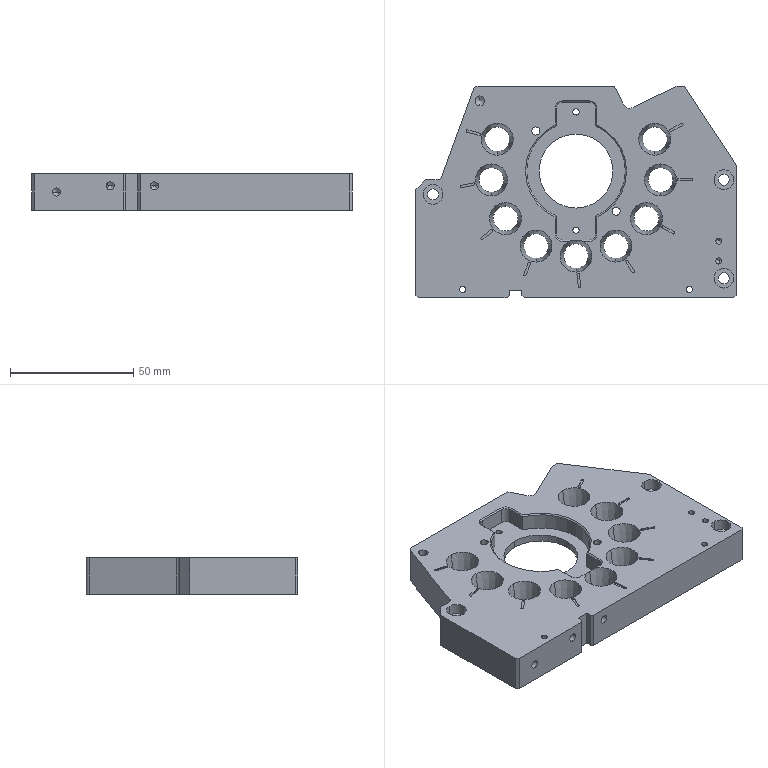NC program | NX | posted with a generic post | part box 130 x 86 x 15 mm
Lines 3649 to 3982 of 51277:
(HOLE_MILLING_COPY , TOOL : D6)
N7254 T06 M6
N7256 G54
N7258 G17 G0 G90 X-1. Y58. B0. C0. S5500 M3
N7260 G43 Z30. H6
N7262 Z0.5
N7264 G94 G3 X-1.5 Y57.5 R0.5 F1500.
N7266 X-1. Y57. R0.5
N7268 X-1. Y57. Z0.4 I0. J1.
N7270 X-1. Y57. Z0.3 I0. J1.
N7272 X-1. Y57. Z0.2 I0. J1.
N7274 X-1. Y57. Z0.1 I0. J1.
N7276 X-1. Y57. Z0. I0. J1.
N7278 X-1. Y57. Z-0.1 I0. J1.
N7280 X-1. Y57. Z-0.2 I0. J1.
N7282 X-1. Y57. Z-0.3 I0. J1.
N7284 X-1. Y57. Z-0.4 I0. J1.
N7286 X-1. Y57. Z-0.5 I0. J1.
N7288 X-1. Y57. Z-0.6 I0. J1.
N7290 X-1. Y57. Z-0.7 I0. J1.
N7292 X-1. Y57. Z-0.8 I0. J1.
N7294 X-1. Y57. Z-0.9 I0. J1.
N7296 X-1. Y57. Z-1. I0. J1.
N7298 X-1. Y57. Z-1.1 I0. J1.
N7300 X-1. Y57. Z-1.2 I0. J1.
N7302 X-1. Y57. Z-1.3 I0. J1.
N7304 X-1. Y57. Z-1.4 I0. J1.
N7306 X-1. Y57. Z-1.5 I0. J1.
N7308 X-1. Y57. Z-1.6 I0. J1.
N7310 X-1. Y57. Z-1.7 I0. J1.
N7312 X-1. Y57. Z-1.8 I0. J1.
N7314 X-1. Y57. Z-1.9 I0. J1.
N7316 X-1. Y57. Z-2. I0. J1.
N7318 X-1. Y57. Z-2.1 I0. J1.
N7320 X-1. Y57. Z-2.2 I0. J1.
N7322 X-1. Y57. Z-2.3 I0. J1.
N7324 X-1. Y57. Z-2.4 I0. J1.
N7326 X-1. Y57. Z-2.5 I0. J1.
N7328 X-1. Y57. Z-2.6 I0. J1.
N7330 X-1. Y57. Z-2.7 I0. J1.
N7332 X-1. Y57. Z-2.8 I0. J1.
N7334 X-1. Y57. Z-2.9 I0. J1.
N7336 X-1. Y57. Z-3. I0. J1.
N7338 X-1. Y57. Z-3.1 I0. J1.
N7340 X-1. Y57. Z-3.2 I0. J1.
N7342 X-1. Y57. Z-3.3 I0. J1.
N7344 X-1. Y57. Z-3.4 I0. J1.
N7346 X-1. Y57. Z-3.5 I0. J1.
N7348 X-1. Y57. Z-3.6 I0. J1.
N7350 X-1. Y57. Z-3.7 I0. J1.
N7352 X-1. Y57. Z-3.8 I0. J1.
N7354 X-1. Y57. Z-3.9 I0. J1.
N7356 X-1. Y57. Z-4. I0. J1.
N7358 X-1. Y57. Z-4.1 I0. J1.
N7360 X-1. Y57. Z-4.2 I0. J1.
N7362 X-1. Y57. Z-4.3 I0. J1.
N7364 X-1. Y57. Z-4.4 I0. J1.
N7366 X-1. Y57. Z-4.5 I0. J1.
N7368 X-1. Y57. Z-4.6 I0. J1.
N7370 X0. Y58. R1.
N7372 X-1. Y57. R-1.
N7374 X-0.5 Y57.5 R0.5
N7376 X-1. Y58. R0.5
N7378 G0 Z30.
N7380 X5. Y-60.
N7382 Z0.5
N7384 G3 X4.5 Y-60.5 R0.5
N7386 X5. Y-61. R0.5
N7388 X5. Y-61. Z0.4 I0. J1.
N7390 X5. Y-61. Z0.3 I0. J1.
N7392 X5. Y-61. Z0.2 I0. J1.
N7394 X5. Y-61. Z0.1 I0. J1.
N7396 X5. Y-61. Z0. I0. J1.
N7398 X5. Y-61. Z-0.1 I0. J1.
N7400 X5. Y-61. Z-0.2 I0. J1.
N7402 X5. Y-61. Z-0.3 I0. J1.
N7404 X5. Y-61. Z-0.4 I0. J1.
N7406 X5. Y-61. Z-0.5 I0. J1.
N7408 X5. Y-61. Z-0.6 I0. J1.
N7410 X5. Y-61. Z-0.7 I0. J1.
N7412 X5. Y-61. Z-0.8 I0. J1.
N7414 X5. Y-61. Z-0.9 I0. J1.
N7416 X5. Y-61. Z-1. I0. J1.
N7418 X5. Y-61. Z-1.1 I0. J1.
N7420 X5. Y-61. Z-1.2 I0. J1.
N7422 X5. Y-61. Z-1.3 I0. J1.
N7424 X5. Y-61. Z-1.4 I0. J1.
N7426 X5. Y-61. Z-1.5 I0. J1.
N7428 X5. Y-61. Z-1.6 I0. J1.
N7430 X5. Y-61. Z-1.7 I0. J1.
N7432 X5. Y-61. Z-1.8 I0. J1.
N7434 X5. Y-61. Z-1.9 I0. J1.
N7436 X5. Y-61. Z-2. I0. J1.
N7438 X5. Y-61. Z-2.1 I0. J1.
N7440 X5. Y-61. Z-2.2 I0. J1.
N7442 X5. Y-61. Z-2.3 I0. J1.
N7444 X5. Y-61. Z-2.4 I0. J1.
N7446 X5. Y-61. Z-2.5 I0. J1.
N7448 X5. Y-61. Z-2.6 I0. J1.
N7450 X5. Y-61. Z-2.7 I0. J1.
N7452 X5. Y-61. Z-2.8 I0. J1.
N7454 X5. Y-61. Z-2.9 I0. J1.
N7456 X5. Y-61. Z-3. I0. J1.
N7458 X5. Y-61. Z-3.1 I0. J1.
N7460 X5. Y-61. Z-3.2 I0. J1.
N7462 X5. Y-61. Z-3.3 I0. J1.
N7464 X5. Y-61. Z-3.4 I0. J1.
N7466 X5. Y-61. Z-3.5 I0. J1.
N7468 X5. Y-61. Z-3.6 I0. J1.
N7470 X5. Y-61. Z-3.7 I0. J1.
N7472 X5. Y-61. Z-3.8 I0. J1.
N7474 X5. Y-61. Z-3.9 I0. J1.
N7476 X5. Y-61. Z-4. I0. J1.
N7478 X5. Y-61. Z-4.1 I0. J1.
N7480 X5. Y-61. Z-4.2 I0. J1.
N7482 X5. Y-61. Z-4.3 I0. J1.
N7484 X5. Y-61. Z-4.4 I0. J1.
N7486 X5. Y-61. Z-4.5 I0. J1.
N7488 X5. Y-61. Z-4.6 I0. J1.
N7490 X6. Y-60. R1.
N7492 X5. Y-61. R-1.
N7494 X5.5 Y-60.5 R0.5
N7496 X5. Y-60. R0.5
N7498 G0 Z30.
N7500 X-35.
N7502 Z0.5
N7504 G3 X-35.5 Y-60.5 R0.5
N7506 X-35. Y-61. R0.5
N7508 X-35. Y-61. Z0.4 I0. J1.
N7510 X-35. Y-61. Z0.3 I0. J1.
N7512 X-35. Y-61. Z0.2 I0. J1.
N7514 X-35. Y-61. Z0.1 I0. J1.
N7516 X-35. Y-61. Z0. I0. J1.
N7518 X-35. Y-61. Z-0.1 I0. J1.
N7520 X-35. Y-61. Z-0.2 I0. J1.
N7522 X-35. Y-61. Z-0.3 I0. J1.
N7524 X-35. Y-61. Z-0.4 I0. J1.
N7526 X-35. Y-61. Z-0.5 I0. J1.
N7528 X-35. Y-61. Z-0.6 I0. J1.
N7530 X-35. Y-61. Z-0.7 I0. J1.
N7532 X-35. Y-61. Z-0.8 I0. J1.
N7534 X-35. Y-61. Z-0.9 I0. J1.
N7536 X-35. Y-61. Z-1. I0. J1.
N7538 X-35. Y-61. Z-1.1 I0. J1.
N7540 X-35. Y-61. Z-1.2 I0. J1.
N7542 X-35. Y-61. Z-1.3 I0. J1.
N7544 X-35. Y-61. Z-1.4 I0. J1.
N7546 X-35. Y-61. Z-1.5 I0. J1.
N7548 X-35. Y-61. Z-1.6 I0. J1.
N7550 X-35. Y-61. Z-1.7 I0. J1.
N7552 X-35. Y-61. Z-1.8 I0. J1.
N7554 X-35. Y-61. Z-1.9 I0. J1.
N7556 X-35. Y-61. Z-2. I0. J1.
N7558 X-35. Y-61. Z-2.1 I0. J1.
N7560 X-35. Y-61. Z-2.2 I0. J1.
N7562 X-35. Y-61. Z-2.3 I0. J1.
N7564 X-35. Y-61. Z-2.4 I0. J1.
N7566 X-35. Y-61. Z-2.5 I0. J1.
N7568 X-35. Y-61. Z-2.6 I0. J1.
N7570 X-35. Y-61. Z-2.7 I0. J1.
N7572 X-35. Y-61. Z-2.8 I0. J1.
N7574 X-35. Y-61. Z-2.9 I0. J1.
N7576 X-35. Y-61. Z-3. I0. J1.
N7578 X-35. Y-61. Z-3.1 I0. J1.
N7580 X-35. Y-61. Z-3.2 I0. J1.
N7582 X-35. Y-61. Z-3.3 I0. J1.
N7584 X-35. Y-61. Z-3.4 I0. J1.
N7586 X-35. Y-61. Z-3.5 I0. J1.
N7588 X-35. Y-61. Z-3.6 I0. J1.
N7590 X-35. Y-61. Z-3.7 I0. J1.
N7592 X-35. Y-61. Z-3.8 I0. J1.
N7594 X-35. Y-61. Z-3.9 I0. J1.
N7596 X-35. Y-61. Z-4. I0. J1.
N7598 X-35. Y-61. Z-4.1 I0. J1.
N7600 X-35. Y-61. Z-4.2 I0. J1.
N7602 X-35. Y-61. Z-4.3 I0. J1.
N7604 X-35. Y-61. Z-4.4 I0. J1.
N7606 X-35. Y-61. Z-4.5 I0. J1.
N7608 X-35. Y-61. Z-4.6 I0. J1.
N7610 X-34. Y-60. R1.
N7612 X-35. Y-61. R-1.
N7614 X-34.5 Y-60.5 R0.5
N7616 X-35. Y-60. R0.5
N7618 G0 Z30.
N7620 M5
(FLOOR_WALL_1_COPY , TOOL : D6JING)
N7622 T16 M6
N7624 G54
N7626 G17 G0 G90 X33.097 Y0.495 B0. C0. S7500 M3
N7628 G43 Z30. H16
N7630 Z-5.9
N7632 G94 G1 Y4.6 Z-7. F1000.
N7634 Y-4.6 F1200.
N7636 X30.203
N7638 Y4.6
N7640 X27.309
N7642 Y-4.6
N7644 X24.801
N7646 G3 X24.526 Y-4.78 R0.3
N7648 G1 X24.415 Y-5.034
N7650 Y5.034
N7652 X23.714 Y6.64
N7654 G3 X21.521 Y10.296 R16.6
N7656 G1 Y-10.296
N7658 G2 X18.627 Y-13.153 R16.6
N7660 G1 Y13.153
N7662 G3 X15.733 Y14.941 R16.6
N7664 G1 Y-14.941
N7666 G2 X12.839 Y-16.023 R16.6
N7668 G1 Y16.023
N7670 G3 X9.945 Y16.537 R16.6
N7672 G1 Y-16.537
N7674 G2 X7.052 Y-16.537 R16.6
N7676 G1 Y16.537
N7678 G3 X4.158 Y16.022 R16.6
N7680 G1 Y-16.022
N7682 G2 X1.264 Y-14.94 R16.6
N7684 G1 Y14.94
N7686 G3 X-1.63 Y13.151 R16.6
N7688 G1 Y-13.151
N7690 G2 X-4.524 Y-10.292 R16.6
N7692 G1 Y10.292
N7694 G3 X-6.714 Y6.64 R16.6
N7696 G1 X-7.418 Y5.027
N7698 Y-5.027
N7700 X-7.526 Y-4.78
N7702 G3 X-7.801 Y-4.6 R0.3
N7704 G1 X-10.312
N7706 Y4.6
N7708 X-13.206
N7710 Y-4.6
N7712 X-16.1
N7714 Y4.6
N7716 Y3.9
N7718 Y4.9 F1000.
N7720 X-16.4 F1200.
N7722 Y-4.9
N7724 X-7.801
N7726 X-6.989 Y-6.76
N7728 G3 X23.989 Y-6.76 R16.9
N7730 G1 X24.801 Y-4.9
N7732 X33.4
N7734 Y4.9
N7736 X24.801
N7738 X23.989 Y6.76
N7740 G3 X-6.989 Y6.76 R16.9
N7742 G1 X-7.801 Y4.9
N7744 X-16.1
N7746 Y3.9
N7748 X-15.4
N7750 Z-6.
N7752 G0 Z30.
(ZLEVEL_PROFILE_2 , TOOL : D6JING)
N7754 X48.353 Y-17.626
N7756 Z-14.
N7758 G1 Z-15. F1000.
N7760 X47.538 Y-17.077
N7762 G3 X46.94 Y-17.035 R0.6
N7764 G1 X44.35 Y-18.299
N7766 X37.085 Y-21.842
N7768 X37.028 Y-21.853
N7770 X37.009 Y-21.908
N7772 X37.047 Y-21.952
N7774 X45.696 Y-39.685
N7776 G2 X45.97 Y-41.424 R3.
N7778 G1 X45.997 Y-41.465
N7780 X46. Y-41.8
N7782 Y-43.46
N7784 G2 X44.195 Y-46.804 R4.
N7786 G1 X13.146 Y-67.18
N7788 G2 X10.402 Y-68. R5.
N7790 G1 X10.035
N7792 X7.655 Y-67.999
N7794 G3 X7.135 Y-68.299 R0.6
N7796 G1 X6.614 Y-69.2
N7798 Z-14.
N7800 G0 Z30.
N7802 X1.041 Y70.804
N7804 Z-14.
N7806 G1 Z-15.
N7808 X0.792 Y69.874
N7810 G3 X0.947 Y69.295 R0.6
N7812 G1 X3.914 Y66.328
N7814 X7.121 Y63.121
N7816 G2 X8. Y61. R3.
N7818 G1 Y57.101
N7820 X42.71 Y44.467
N7822 G2 X46. Y39.769 R5.
N7824 G1 Y39.358
N7826 X45.999 Y36.99
N7828 G3 X46.299 Y36.47 R0.6
N7830 G1 X47.2 Y35.95
N7832 Z-14.
N7834 G0 Z30.
(ZLEVEL_PROFILE_2_COPY , TOOL : D6JING)
N7836 X22.995 Y-3.833
N7838 Z-6.
N7840 G1 Z-7.
N7842 X23.496 Y-4.7
N7844 G3 X24.015 Y-5. R0.6
N7846 G1 X27.546
N7848 X33.5
N7850 Y5.
N7852 X27.546
N7854 X24.015
N7856 G3 X23.496 Y4.7 R0.6
N7858 G1 X22.996 Y3.833
N7860 Z-6.
N7862 G0 Z30.
N7864 X-5.998 Y3.838
N7866 Z-6.
N7868 G1 Z-7.
N7870 X-6.496 Y4.7
N7872 G3 X-7.015 Y5. R0.6
N7874 G1 X-9.862
N7876 X-16.5
N7878 Y-5.
N7880 X-9.83
N7882 X-9.268 Y-5.053
N7884 X-9.222 Y-5.
N7886 X-7.015
N7888 G3 X-6.496 Y-4.7 R0.6
N7890 G1 X-5.996 Y-3.835
N7892 Z-6.
N7894 G0 Z30.
N7896 M5